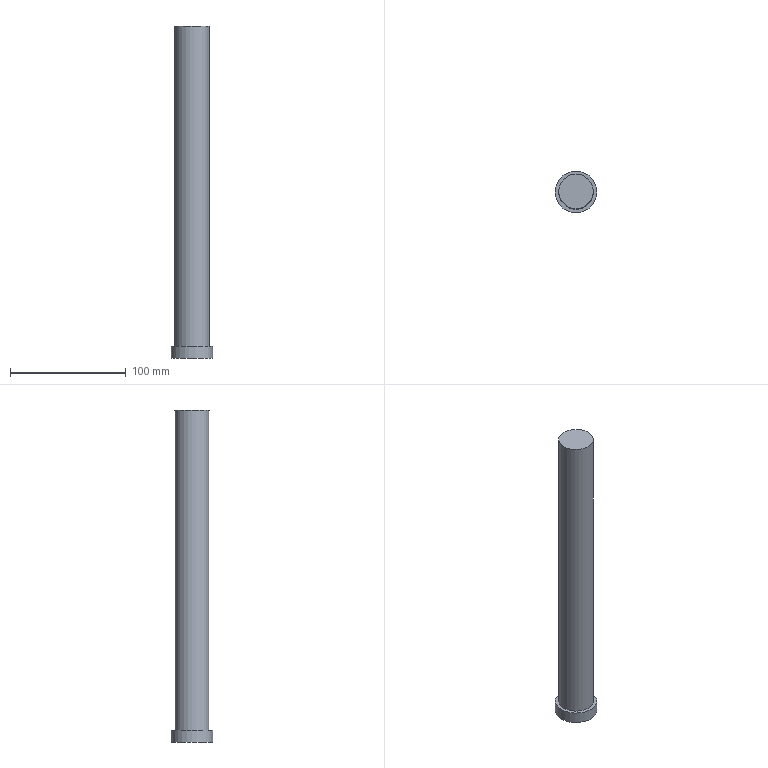Part | STEP file | RP-D30-287L | 1 solid | 5 faces | box 36 x 36 x 287 mm | volume 205979 mm3 | plane 3 | cylinder 2 | commonest cylinder face diameters 30 x1 36 x1
STEP:
#1=CARTESIAN_POINT('',(0.,0.,0.));
#2=DIRECTION('',(0.,0.,1.));
#3=DIRECTION('',(1.,0.,0.));
#4=AXIS2_PLACEMENT_3D('',#1,#2,#3);
#5=CARTESIAN_POINT('',(153.,-292.,21.));
#6=VERTEX_POINT('',#5);
#7=CARTESIAN_POINT('',(123.,-292.,21.));
#8=VERTEX_POINT('',#7);
#9=CARTESIAN_POINT('',(138.,-292.,21.));
#10=DIRECTION('',(0.,0.,1.));
#11=DIRECTION('',(-1.,0.,0.));
#12=AXIS2_PLACEMENT_3D('',#9,#10,#11);
#13=CIRCLE('',#12,15.);
#14=CARTESIAN_POINT('',(138.,-292.,539.));
#15=DIRECTION('',(0.,0.,-1.));
#16=DIRECTION('',(1.,0.,0.));
#17=AXIS2_PLACEMENT_3D('',#14,#15,#16);
#18=CYLINDRICAL_SURFACE('',#17,15.);
#19=CARTESIAN_POINT('',(9.425,518.));
#20=DIRECTION('',(-1.,0.));
#21=VECTOR('',#20,1.);
#22=LINE('',#19,#21);
#23=(GEOMETRIC_REPRESENTATION_CONTEXT(2)PARAMETRIC_REPRESENTATION_CONTEXT()REPRESENTATION_CONTEXT('',''));
#24=DEFINITIONAL_REPRESENTATION('',(#22),#23);
#25=PCURVE('',#18,#24);
#26=CARTESIAN_POINT('',(-275.,-325.,21.));
#27=DIRECTION('',(0.,0.,1.));
#28=DIRECTION('',(-1.,0.,0.));
#29=AXIS2_PLACEMENT_3D('',#26,#27,#28);
#30=PLANE('',#29);
#31=CARTESIAN_POINT('',(-413.,-33.));
#32=DIRECTION('',(1.,0.));
#33=AXIS2_PLACEMENT_2D('',#31,#32);
#34=CIRCLE('',#33,15.);
#35=(GEOMETRIC_REPRESENTATION_CONTEXT(2)PARAMETRIC_REPRESENTATION_CONTEXT()REPRESENTATION_CONTEXT('',''));
#36=DEFINITIONAL_REPRESENTATION('',(#34),#35);
#37=PCURVE('',#30,#36);
#38=SURFACE_CURVE('',#13,(#25,#37),.PCURVE_S1.);
#39=EDGE_CURVE('',#6,#8,#38,.T.);
#40=ORIENTED_EDGE('',*,*,#39,.F.);
#41=CARTESIAN_POINT('',(153.,-292.,-256.));
#42=VERTEX_POINT('',#41);
#43=CARTESIAN_POINT('',(153.,-292.,21.));
#44=CARTESIAN_POINT('',(153.,-292.,-256.));
#45=B_SPLINE_CURVE_WITH_KNOTS('',1,(#43,#44),.UNSPECIFIED.,.F.,.F.,(2,2),(518.,795.),.PIECEWISE_BEZIER_KNOTS.);
#46=CARTESIAN_POINT('',(6.283,0.));
#47=DIRECTION('',(0.,1.));
#48=VECTOR('',#47,1.);
#49=LINE('',#46,#48);
#50=(GEOMETRIC_REPRESENTATION_CONTEXT(2)PARAMETRIC_REPRESENTATION_CONTEXT()REPRESENTATION_CONTEXT('',''));
#51=DEFINITIONAL_REPRESENTATION('',(#49),#50);
#52=PCURVE('',#18,#51);
#53=CARTESIAN_POINT('',(0.,0.));
#54=DIRECTION('',(0.,1.));
#55=VECTOR('',#54,1.);
#56=LINE('',#53,#55);
#57=(GEOMETRIC_REPRESENTATION_CONTEXT(2)PARAMETRIC_REPRESENTATION_CONTEXT()REPRESENTATION_CONTEXT('',''));
#58=DEFINITIONAL_REPRESENTATION('',(#56),#57);
#59=PCURVE('',#18,#58);
#60=SEAM_CURVE('',#45,(#52,#59),.PCURVE_S1.);
#61=EDGE_CURVE('',#6,#42,#60,.T.);
#62=ORIENTED_EDGE('',*,*,#61,.T.);
#63=CARTESIAN_POINT('',(138.,-292.,-256.));
#64=DIRECTION('',(0.,0.,-1.));
#65=DIRECTION('',(1.,0.,0.));
#66=AXIS2_PLACEMENT_3D('',#63,#64,#65);
#67=CIRCLE('',#66,15.);
#68=CARTESIAN_POINT('',(0.,795.));
#69=DIRECTION('',(1.,0.));
#70=VECTOR('',#69,1.);
#71=LINE('',#68,#70);
#72=(GEOMETRIC_REPRESENTATION_CONTEXT(2)PARAMETRIC_REPRESENTATION_CONTEXT()REPRESENTATION_CONTEXT('',''));
#73=DEFINITIONAL_REPRESENTATION('',(#71),#72);
#74=PCURVE('',#18,#73);
#75=CARTESIAN_POINT('',(138.,-292.,-256.));
#76=DIRECTION('',(0.,0.,-1.));
#77=DIRECTION('',(1.,0.,0.));
#78=AXIS2_PLACEMENT_3D('',#75,#76,#77);
#79=PLANE('',#78);
#80=CARTESIAN_POINT('',(0.,0.));
#81=DIRECTION('',(1.,0.));
#82=AXIS2_PLACEMENT_2D('',#80,#81);
#83=CIRCLE('',#82,15.);
#84=(GEOMETRIC_REPRESENTATION_CONTEXT(2)PARAMETRIC_REPRESENTATION_CONTEXT()REPRESENTATION_CONTEXT('',''));
#85=DEFINITIONAL_REPRESENTATION('',(#83),#84);
#86=PCURVE('',#79,#85);
#87=SURFACE_CURVE('',#67,(#74,#86),.PCURVE_S1.);
#88=EDGE_CURVE('',#42,#42,#87,.T.);
#89=ORIENTED_EDGE('',*,*,#88,.F.);
#90=ORIENTED_EDGE('',*,*,#61,.F.);
#91=CARTESIAN_POINT('',(138.,-292.,21.));
#92=DIRECTION('',(0.,0.,1.));
#93=DIRECTION('',(-1.,0.,0.));
#94=AXIS2_PLACEMENT_3D('',#91,#92,#93);
#95=CIRCLE('',#94,15.);
#96=CARTESIAN_POINT('',(3.142,518.));
#97=DIRECTION('',(-1.,0.));
#98=VECTOR('',#97,1.);
#99=LINE('',#96,#98);
#100=(GEOMETRIC_REPRESENTATION_CONTEXT(2)PARAMETRIC_REPRESENTATION_CONTEXT()REPRESENTATION_CONTEXT('',''));
#101=DEFINITIONAL_REPRESENTATION('',(#99),#100);
#102=PCURVE('',#18,#101);
#103=CARTESIAN_POINT('',(-413.,-33.));
#104=DIRECTION('',(1.,0.));
#105=AXIS2_PLACEMENT_2D('',#103,#104);
#106=CIRCLE('',#105,15.);
#107=(GEOMETRIC_REPRESENTATION_CONTEXT(2)PARAMETRIC_REPRESENTATION_CONTEXT()REPRESENTATION_CONTEXT('',''));
#108=DEFINITIONAL_REPRESENTATION('',(#106),#107);
#109=PCURVE('',#30,#108);
#110=SURFACE_CURVE('',#95,(#102,#109),.PCURVE_S1.);
#111=EDGE_CURVE('',#8,#6,#110,.T.);
#112=ORIENTED_EDGE('',*,*,#111,.F.);
#113=EDGE_LOOP('',(#40,#62,#89,#90,#112));
#114=FACE_BOUND('',#113,.T.);
#115=ADVANCED_FACE('',(#114),#18,.T.);
#116=ORIENTED_EDGE('',*,*,#111,.T.);
#117=ORIENTED_EDGE('',*,*,#39,.T.);
#118=EDGE_LOOP('',(#116,#117));
#119=FACE_BOUND('',#118,.T.);
#120=ADVANCED_FACE('',(#119),#30,.T.);
#121=CARTESIAN_POINT('',(156.,-292.,-266.));
#122=VERTEX_POINT('',#121);
#123=CARTESIAN_POINT('',(138.,-292.,-266.));
#124=DIRECTION('',(0.,0.,1.));
#125=DIRECTION('',(1.,0.,0.));
#126=AXIS2_PLACEMENT_3D('',#123,#124,#125);
#127=CIRCLE('',#126,18.);
#128=CARTESIAN_POINT('',(138.,-292.,-266.));
#129=DIRECTION('',(0.,0.,1.));
#130=DIRECTION('',(-1.,0.,0.));
#131=AXIS2_PLACEMENT_3D('',#128,#129,#130);
#132=CYLINDRICAL_SURFACE('',#131,18.);
#133=CARTESIAN_POINT('',(3.142,0.));
#134=DIRECTION('',(1.,0.));
#135=VECTOR('',#134,1.);
#136=LINE('',#133,#135);
#137=(GEOMETRIC_REPRESENTATION_CONTEXT(2)PARAMETRIC_REPRESENTATION_CONTEXT()REPRESENTATION_CONTEXT('',''));
#138=DEFINITIONAL_REPRESENTATION('',(#136),#137);
#139=PCURVE('',#132,#138);
#140=CARTESIAN_POINT('',(185.,-325.,-266.));
#141=DIRECTION('',(0.,0.,1.));
#142=DIRECTION('',(-1.,0.,0.));
#143=AXIS2_PLACEMENT_3D('',#140,#141,#142);
#144=PLANE('',#143);
#145=CARTESIAN_POINT('',(47.,-33.));
#146=DIRECTION('',(-1.,0.));
#147=AXIS2_PLACEMENT_2D('',#145,#146);
#148=CIRCLE('',#147,18.);
#149=(GEOMETRIC_REPRESENTATION_CONTEXT(2)PARAMETRIC_REPRESENTATION_CONTEXT()REPRESENTATION_CONTEXT('',''));
#150=DEFINITIONAL_REPRESENTATION('',(#148),#149);
#151=PCURVE('',#144,#150);
#152=SURFACE_CURVE('',#127,(#139,#151),.PCURVE_S1.);
#153=EDGE_CURVE('',#122,#122,#152,.T.);
#154=ORIENTED_EDGE('',*,*,#153,.T.);
#155=CARTESIAN_POINT('',(156.,-292.,-256.));
#156=VERTEX_POINT('',#155);
#157=CARTESIAN_POINT('',(156.,-292.,-266.));
#158=CARTESIAN_POINT('',(156.,-292.,-256.));
#159=B_SPLINE_CURVE_WITH_KNOTS('',1,(#157,#158),.UNSPECIFIED.,.F.,.F.,(2,2),(0.,10.),.PIECEWISE_BEZIER_KNOTS.);
#160=CARTESIAN_POINT('',(9.425,0.));
#161=DIRECTION('',(0.,1.));
#162=VECTOR('',#161,1.);
#163=LINE('',#160,#162);
#164=(GEOMETRIC_REPRESENTATION_CONTEXT(2)PARAMETRIC_REPRESENTATION_CONTEXT()REPRESENTATION_CONTEXT('',''));
#165=DEFINITIONAL_REPRESENTATION('',(#163),#164);
#166=PCURVE('',#132,#165);
#167=CARTESIAN_POINT('',(3.142,0.));
#168=DIRECTION('',(0.,1.));
#169=VECTOR('',#168,1.);
#170=LINE('',#167,#169);
#171=(GEOMETRIC_REPRESENTATION_CONTEXT(2)PARAMETRIC_REPRESENTATION_CONTEXT()REPRESENTATION_CONTEXT('',''));
#172=DEFINITIONAL_REPRESENTATION('',(#170),#171);
#173=PCURVE('',#132,#172);
#174=SEAM_CURVE('',#159,(#166,#173),.PCURVE_S1.);
#175=EDGE_CURVE('',#122,#156,#174,.T.);
#176=ORIENTED_EDGE('',*,*,#175,.T.);
#177=CARTESIAN_POINT('',(138.,-292.,-256.));
#178=DIRECTION('',(0.,0.,1.));
#179=DIRECTION('',(1.,0.,0.));
#180=AXIS2_PLACEMENT_3D('',#177,#178,#179);
#181=CIRCLE('',#180,18.);
#182=CARTESIAN_POINT('',(3.142,10.));
#183=DIRECTION('',(1.,0.));
#184=VECTOR('',#183,1.);
#185=LINE('',#182,#184);
#186=(GEOMETRIC_REPRESENTATION_CONTEXT(2)PARAMETRIC_REPRESENTATION_CONTEXT()REPRESENTATION_CONTEXT('',''));
#187=DEFINITIONAL_REPRESENTATION('',(#185),#186);
#188=PCURVE('',#132,#187);
#189=CARTESIAN_POINT('',(18.,0.));
#190=CARTESIAN_POINT('',(18.,-31.177));
#191=CARTESIAN_POINT('',(-9.,-15.588));
#192=CARTESIAN_POINT('',(-36.,0.));
#193=CARTESIAN_POINT('',(-9.,15.588));
#194=CARTESIAN_POINT('',(18.,31.177));
#195=CARTESIAN_POINT('',(18.,0.));
#196=(BOUNDED_CURVE()B_SPLINE_CURVE(2,(#189,#190,#191,#192,#193,#194,#195),.UNSPECIFIED.,.T.,.F.)B_SPLINE_CURVE_WITH_KNOTS((1,2,2,2,2,1),(-2.094,0.,2.094,4.189,6.283,8.378),.UNSPECIFIED.)CURVE()GEOMETRIC_REPRESENTATION_ITEM()RATIONAL_B_SPLINE_CURVE((1.,0.5,1.,0.5,1.,0.5,1.))REPRESENTATION_ITEM(''));
#197=(GEOMETRIC_REPRESENTATION_CONTEXT(2)PARAMETRIC_REPRESENTATION_CONTEXT()REPRESENTATION_CONTEXT('',''));
#198=DEFINITIONAL_REPRESENTATION('',(#196),#197);
#199=PCURVE('',#79,#198);
#200=SURFACE_CURVE('',#181,(#188,#199),.PCURVE_S1.);
#201=EDGE_CURVE('',#156,#156,#200,.T.);
#202=ORIENTED_EDGE('',*,*,#201,.F.);
#203=ORIENTED_EDGE('',*,*,#175,.F.);
#204=EDGE_LOOP('',(#154,#176,#202,#203));
#205=FACE_BOUND('',#204,.T.);
#206=ADVANCED_FACE('',(#205),#132,.T.);
#207=ORIENTED_EDGE('',*,*,#88,.T.);
#208=EDGE_LOOP('',(#207));
#209=FACE_BOUND('',#208,.T.);
#210=ORIENTED_EDGE('',*,*,#201,.T.);
#211=EDGE_LOOP('',(#210));
#212=FACE_BOUND('',#211,.T.);
#213=ADVANCED_FACE('',(#209,#212),#79,.F.);
#214=ORIENTED_EDGE('',*,*,#153,.F.);
#215=EDGE_LOOP('',(#214));
#216=FACE_BOUND('',#215,.T.);
#217=ADVANCED_FACE('',(#216),#144,.F.);
#218=CLOSED_SHELL('',(#115,#120,#206,#213,#217));
#219=MANIFOLD_SOLID_BREP('',#218);
#220=(LENGTH_UNIT()NAMED_UNIT(*)SI_UNIT(.MILLI.,.METRE.));
#221=UNCERTAINTY_MEASURE_WITH_UNIT(LENGTH_MEASURE(0.000005),#220,'','');
#222=(NAMED_UNIT(*)PLANE_ANGLE_UNIT()SI_UNIT($,.RADIAN.));
#223=(NAMED_UNIT(*)SI_UNIT($,.STERADIAN.)SOLID_ANGLE_UNIT());
#224=(GEOMETRIC_REPRESENTATION_CONTEXT(3)GLOBAL_UNCERTAINTY_ASSIGNED_CONTEXT((#221))GLOBAL_UNIT_ASSIGNED_CONTEXT((#220,#222,#223))REPRESENTATION_CONTEXT('',''));
#225=ADVANCED_BREP_SHAPE_REPRESENTATION('',(#4,#219),#224);